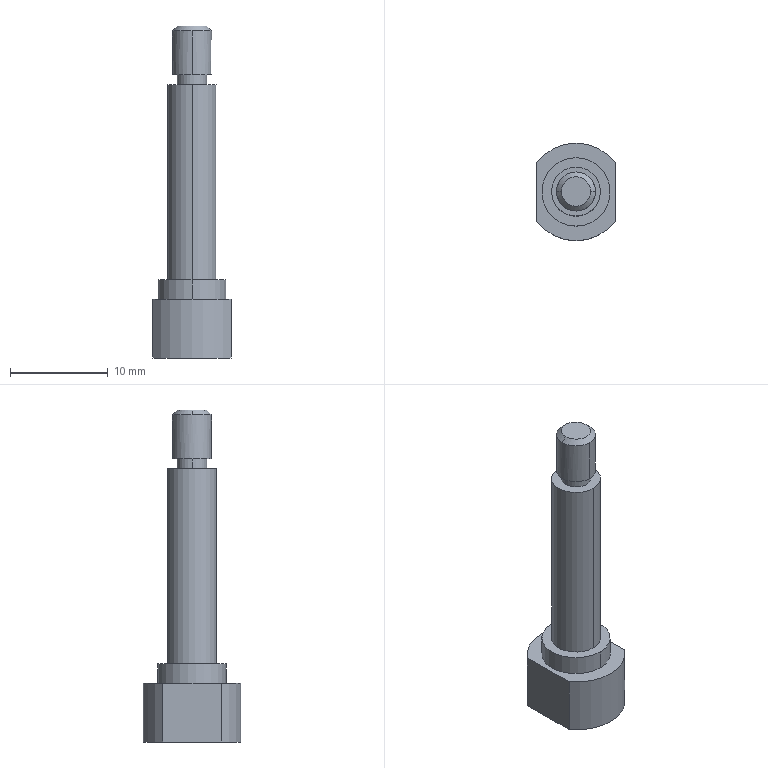Part | STEP file | 06-10 Guide mixing wheel support shaft | 1 solid | 24 faces | box 8 x 10 x 34 mm | volume 879.659 mm3 | cylinder 12 | plane 8 | cone 4 | commonest cylinder face diameters 3 x2 3.3 x2 4 x2 5 x2 7 x2 10 x2